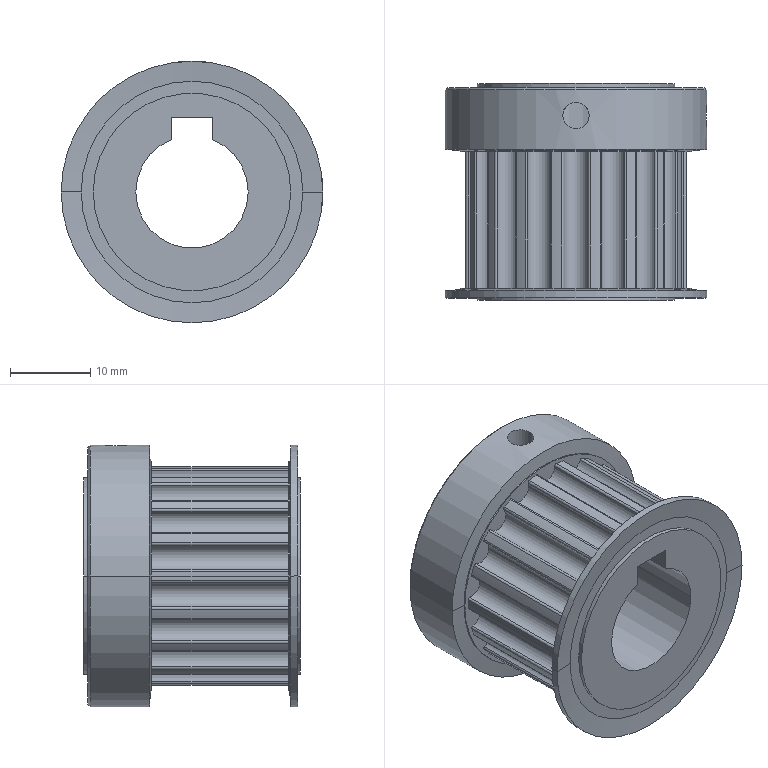Part | STEP file | 1 solid | 109 faces | box 32.58 x 27 x 32.58 mm | volume 11988 mm3 | cylinder 92 | plane 9 | cone 8 | commonest cylinder face diameters 0.488 x36 27.5 x19 3 x18 3.3 x4 24.58 x4 28.65 x4